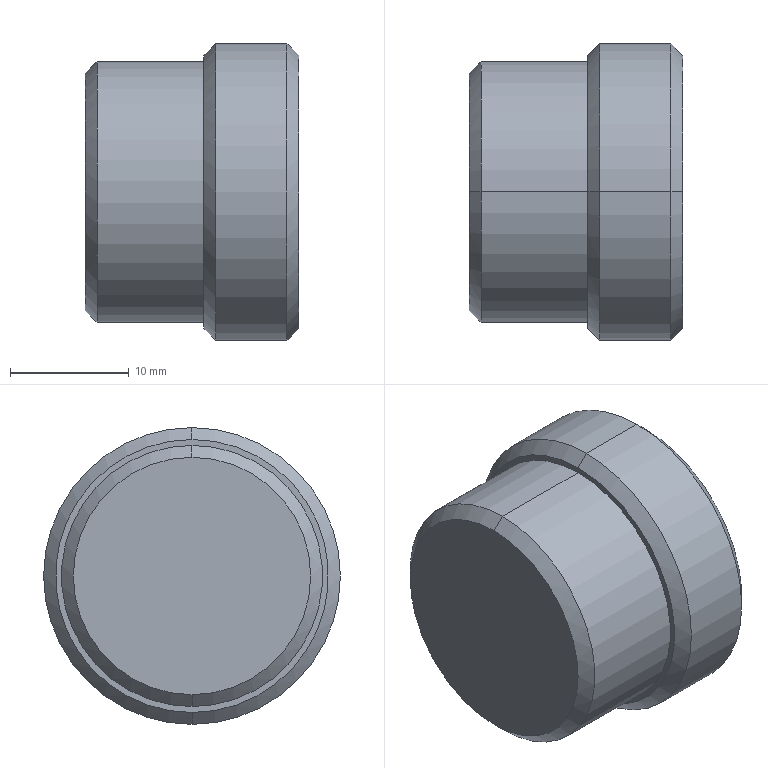Part | STEP file | Panel plug T02 | 1 solid | 13 faces | box 18 x 25 x 25 mm | volume 7618 mm3 | cone 6 | cylinder 4 | plane 3 | commonest cylinder face diameters 22 x2 25 x2
STEP:
#1=CARTESIAN_POINT('',(0.,0.,0.));
#2=DIRECTION('',(0.,0.,1.));
#3=DIRECTION('',(1.,0.,0.));
#4=AXIS2_PLACEMENT_3D('',#1,#2,#3);
#5=CARTESIAN_POINT('',(18.,0.,-11.5));
#6=VERTEX_POINT('',#5);
#7=CARTESIAN_POINT('',(18.,0.,11.5));
#8=VERTEX_POINT('',#7);
#9=CARTESIAN_POINT('',(18.,0.,0.));
#10=DIRECTION('',(1.,0.,0.));
#11=DIRECTION('',(0.,0.,-1.));
#12=AXIS2_PLACEMENT_3D('',#9,#10,#11);
#13=CIRCLE('',#12,11.5);
#14=CARTESIAN_POINT('',(18.,0.,0.));
#15=DIRECTION('',(-1.,0.,0.));
#16=DIRECTION('',(0.,0.,1.));
#17=AXIS2_PLACEMENT_3D('',#14,#15,#16);
#18=CONICAL_SURFACE('',#17,11.5,0.7854);
#19=CARTESIAN_POINT('',(3.142,0.));
#20=DIRECTION('',(-1.,0.));
#21=VECTOR('',#20,1.);
#22=LINE('',#19,#21);
#23=(GEOMETRIC_REPRESENTATION_CONTEXT(2)PARAMETRIC_REPRESENTATION_CONTEXT()REPRESENTATION_CONTEXT('',''));
#24=DEFINITIONAL_REPRESENTATION('',(#22),#23);
#25=PCURVE('',#18,#24);
#26=CARTESIAN_POINT('',(18.,0.,-12.5));
#27=DIRECTION('',(1.,0.,0.));
#28=DIRECTION('',(0.,0.,-1.));
#29=AXIS2_PLACEMENT_3D('',#26,#27,#28);
#30=PLANE('',#29);
#31=CARTESIAN_POINT('',(-12.5,0.));
#32=DIRECTION('',(1.,0.));
#33=AXIS2_PLACEMENT_2D('',#31,#32);
#34=CIRCLE('',#33,11.5);
#35=(GEOMETRIC_REPRESENTATION_CONTEXT(2)PARAMETRIC_REPRESENTATION_CONTEXT()REPRESENTATION_CONTEXT('',''));
#36=DEFINITIONAL_REPRESENTATION('',(#34),#35);
#37=PCURVE('',#30,#36);
#38=SURFACE_CURVE('',#13,(#25,#37),.PCURVE_S1.);
#39=EDGE_CURVE('',#6,#8,#38,.T.);
#40=ORIENTED_EDGE('',*,*,#39,.F.);
#41=CARTESIAN_POINT('',(17.,0.,-12.5));
#42=VERTEX_POINT('',#41);
#43=CARTESIAN_POINT('',(18.,0.,-11.5));
#44=DIRECTION('',(-0.7071,0.,-0.7071));
#45=VECTOR('',#44,1.);
#46=LINE('',#43,#45);
#47=CARTESIAN_POINT('',(3.142,0.));
#48=DIRECTION('',(0.,1.));
#49=VECTOR('',#48,1.);
#50=LINE('',#47,#49);
#51=(GEOMETRIC_REPRESENTATION_CONTEXT(2)PARAMETRIC_REPRESENTATION_CONTEXT()REPRESENTATION_CONTEXT('',''));
#52=DEFINITIONAL_REPRESENTATION('',(#50),#51);
#53=PCURVE('',#18,#52);
#54=CARTESIAN_POINT('',(18.,0.,0.));
#55=DIRECTION('',(-1.,0.,0.));
#56=DIRECTION('',(0.,0.,1.));
#57=AXIS2_PLACEMENT_3D('',#54,#55,#56);
#58=CONICAL_SURFACE('',#57,11.5,0.7854);
#59=CARTESIAN_POINT('',(3.142,0.));
#60=DIRECTION('',(0.,1.));
#61=VECTOR('',#60,1.);
#62=LINE('',#59,#61);
#63=(GEOMETRIC_REPRESENTATION_CONTEXT(2)PARAMETRIC_REPRESENTATION_CONTEXT()REPRESENTATION_CONTEXT('',''));
#64=DEFINITIONAL_REPRESENTATION('',(#62),#63);
#65=PCURVE('',#58,#64);
#66=SURFACE_CURVE('',#46,(#53,#65),.PCURVE_S1.);
#67=EDGE_CURVE('',#6,#42,#66,.T.);
#68=ORIENTED_EDGE('',*,*,#67,.T.);
#69=CARTESIAN_POINT('',(17.,0.,12.5));
#70=VERTEX_POINT('',#69);
#71=CARTESIAN_POINT('',(17.,0.,0.));
#72=DIRECTION('',(-1.,0.,0.));
#73=DIRECTION('',(0.,0.,-1.));
#74=AXIS2_PLACEMENT_3D('',#71,#72,#73);
#75=CIRCLE('',#74,12.5);
#76=CARTESIAN_POINT('',(-3.142,1.));
#77=DIRECTION('',(1.,0.));
#78=VECTOR('',#77,1.);
#79=LINE('',#76,#78);
#80=(GEOMETRIC_REPRESENTATION_CONTEXT(2)PARAMETRIC_REPRESENTATION_CONTEXT()REPRESENTATION_CONTEXT('',''));
#81=DEFINITIONAL_REPRESENTATION('',(#79),#80);
#82=PCURVE('',#18,#81);
#83=CARTESIAN_POINT('',(18.,0.,0.));
#84=DIRECTION('',(1.,0.,0.));
#85=DIRECTION('',(0.,0.,-1.));
#86=AXIS2_PLACEMENT_3D('',#83,#84,#85);
#87=CYLINDRICAL_SURFACE('',#86,12.5);
#88=CARTESIAN_POINT('',(6.283,-1.));
#89=DIRECTION('',(-1.,0.));
#90=VECTOR('',#89,1.);
#91=LINE('',#88,#90);
#92=(GEOMETRIC_REPRESENTATION_CONTEXT(2)PARAMETRIC_REPRESENTATION_CONTEXT()REPRESENTATION_CONTEXT('',''));
#93=DEFINITIONAL_REPRESENTATION('',(#91),#92);
#94=PCURVE('',#87,#93);
#95=SURFACE_CURVE('',#75,(#82,#94),.PCURVE_S1.);
#96=EDGE_CURVE('',#70,#42,#95,.T.);
#97=ORIENTED_EDGE('',*,*,#96,.F.);
#98=CARTESIAN_POINT('',(18.,0.,11.5));
#99=DIRECTION('',(-0.7071,0.,0.7071));
#100=VECTOR('',#99,1.);
#101=LINE('',#98,#100);
#102=CARTESIAN_POINT('',(0.,0.));
#103=DIRECTION('',(0.,1.));
#104=VECTOR('',#103,1.);
#105=LINE('',#102,#104);
#106=(GEOMETRIC_REPRESENTATION_CONTEXT(2)PARAMETRIC_REPRESENTATION_CONTEXT()REPRESENTATION_CONTEXT('',''));
#107=DEFINITIONAL_REPRESENTATION('',(#105),#106);
#108=PCURVE('',#18,#107);
#109=CARTESIAN_POINT('',(6.283,0.));
#110=DIRECTION('',(0.,1.));
#111=VECTOR('',#110,1.);
#112=LINE('',#109,#111);
#113=(GEOMETRIC_REPRESENTATION_CONTEXT(2)PARAMETRIC_REPRESENTATION_CONTEXT()REPRESENTATION_CONTEXT('',''));
#114=DEFINITIONAL_REPRESENTATION('',(#112),#113);
#115=PCURVE('',#58,#114);
#116=SURFACE_CURVE('',#101,(#108,#115),.PCURVE_S1.);
#117=EDGE_CURVE('',#8,#70,#116,.T.);
#118=ORIENTED_EDGE('',*,*,#117,.F.);
#119=EDGE_LOOP('',(#40,#68,#97,#118));
#120=FACE_BOUND('',#119,.T.);
#121=ADVANCED_FACE('',(#120),#18,.T.);
#122=CARTESIAN_POINT('',(10.,0.,11.5));
#123=VERTEX_POINT('',#122);
#124=CARTESIAN_POINT('',(10.,0.,-11.5));
#125=VERTEX_POINT('',#124);
#126=CARTESIAN_POINT('',(10.,0.,0.));
#127=DIRECTION('',(-1.,0.,0.));
#128=DIRECTION('',(0.,0.,1.));
#129=AXIS2_PLACEMENT_3D('',#126,#127,#128);
#130=CIRCLE('',#129,11.5);
#131=CARTESIAN_POINT('',(11.,0.,0.));
#132=DIRECTION('',(1.,0.,0.));
#133=DIRECTION('',(0.,0.,-1.));
#134=AXIS2_PLACEMENT_3D('',#131,#132,#133);
#135=CONICAL_SURFACE('',#134,12.5,0.7854);
#136=CARTESIAN_POINT('',(3.142,-1.));
#137=DIRECTION('',(-1.,0.));
#138=VECTOR('',#137,1.);
#139=LINE('',#136,#138);
#140=(GEOMETRIC_REPRESENTATION_CONTEXT(2)PARAMETRIC_REPRESENTATION_CONTEXT()REPRESENTATION_CONTEXT('',''));
#141=DEFINITIONAL_REPRESENTATION('',(#139),#140);
#142=PCURVE('',#135,#141);
#143=CARTESIAN_POINT('',(10.,0.,-11.));
#144=DIRECTION('',(-1.,0.,0.));
#145=DIRECTION('',(0.,0.,1.));
#146=AXIS2_PLACEMENT_3D('',#143,#144,#145);
#147=PLANE('',#146);
#148=CARTESIAN_POINT('',(11.,0.));
#149=DIRECTION('',(1.,0.));
#150=AXIS2_PLACEMENT_2D('',#148,#149);
#151=CIRCLE('',#150,11.5);
#152=(GEOMETRIC_REPRESENTATION_CONTEXT(2)PARAMETRIC_REPRESENTATION_CONTEXT()REPRESENTATION_CONTEXT('',''));
#153=DEFINITIONAL_REPRESENTATION('',(#151),#152);
#154=PCURVE('',#147,#153);
#155=SURFACE_CURVE('',#130,(#142,#154),.PCURVE_S1.);
#156=EDGE_CURVE('',#123,#125,#155,.T.);
#157=ORIENTED_EDGE('',*,*,#156,.F.);
#158=CARTESIAN_POINT('',(11.,0.,12.5));
#159=VERTEX_POINT('',#158);
#160=CARTESIAN_POINT('',(11.,0.,12.5));
#161=DIRECTION('',(0.7071,0.,0.7071));
#162=VECTOR('',#161,1.);
#163=LINE('',#160,#162);
#164=CARTESIAN_POINT('',(3.142,0.));
#165=DIRECTION('',(0.,1.));
#166=VECTOR('',#165,1.);
#167=LINE('',#164,#166);
#168=(GEOMETRIC_REPRESENTATION_CONTEXT(2)PARAMETRIC_REPRESENTATION_CONTEXT()REPRESENTATION_CONTEXT('',''));
#169=DEFINITIONAL_REPRESENTATION('',(#167),#168);
#170=PCURVE('',#135,#169);
#171=CARTESIAN_POINT('',(11.,0.,0.));
#172=DIRECTION('',(1.,0.,0.));
#173=DIRECTION('',(0.,0.,-1.));
#174=AXIS2_PLACEMENT_3D('',#171,#172,#173);
#175=CONICAL_SURFACE('',#174,12.5,0.7854);
#176=CARTESIAN_POINT('',(3.142,0.));
#177=DIRECTION('',(0.,1.));
#178=VECTOR('',#177,1.);
#179=LINE('',#176,#178);
#180=(GEOMETRIC_REPRESENTATION_CONTEXT(2)PARAMETRIC_REPRESENTATION_CONTEXT()REPRESENTATION_CONTEXT('',''));
#181=DEFINITIONAL_REPRESENTATION('',(#179),#180);
#182=PCURVE('',#175,#181);
#183=SURFACE_CURVE('',#163,(#170,#182),.PCURVE_S1.);
#184=EDGE_CURVE('',#123,#159,#183,.T.);
#185=ORIENTED_EDGE('',*,*,#184,.T.);
#186=CARTESIAN_POINT('',(11.,0.,-12.5));
#187=VERTEX_POINT('',#186);
#188=CARTESIAN_POINT('',(11.,0.,0.));
#189=DIRECTION('',(1.,0.,0.));
#190=DIRECTION('',(0.,0.,1.));
#191=AXIS2_PLACEMENT_3D('',#188,#189,#190);
#192=CIRCLE('',#191,12.5);
#193=CARTESIAN_POINT('',(-3.142,0.));
#194=DIRECTION('',(1.,0.));
#195=VECTOR('',#194,1.);
#196=LINE('',#193,#195);
#197=(GEOMETRIC_REPRESENTATION_CONTEXT(2)PARAMETRIC_REPRESENTATION_CONTEXT()REPRESENTATION_CONTEXT('',''));
#198=DEFINITIONAL_REPRESENTATION('',(#196),#197);
#199=PCURVE('',#135,#198);
#200=CARTESIAN_POINT('',(-3.142,-7.));
#201=DIRECTION('',(1.,0.));
#202=VECTOR('',#201,1.);
#203=LINE('',#200,#202);
#204=(GEOMETRIC_REPRESENTATION_CONTEXT(2)PARAMETRIC_REPRESENTATION_CONTEXT()REPRESENTATION_CONTEXT('',''));
#205=DEFINITIONAL_REPRESENTATION('',(#203),#204);
#206=PCURVE('',#87,#205);
#207=SURFACE_CURVE('',#192,(#199,#206),.PCURVE_S1.);
#208=EDGE_CURVE('',#187,#159,#207,.T.);
#209=ORIENTED_EDGE('',*,*,#208,.F.);
#210=CARTESIAN_POINT('',(11.,0.,-12.5));
#211=DIRECTION('',(0.7071,0.,-0.7071));
#212=VECTOR('',#211,1.);
#213=LINE('',#210,#212);
#214=CARTESIAN_POINT('',(0.,0.));
#215=DIRECTION('',(0.,1.));
#216=VECTOR('',#215,1.);
#217=LINE('',#214,#216);
#218=(GEOMETRIC_REPRESENTATION_CONTEXT(2)PARAMETRIC_REPRESENTATION_CONTEXT()REPRESENTATION_CONTEXT('',''));
#219=DEFINITIONAL_REPRESENTATION('',(#217),#218);
#220=PCURVE('',#135,#219);
#221=CARTESIAN_POINT('',(6.283,0.));
#222=DIRECTION('',(0.,1.));
#223=VECTOR('',#222,1.);
#224=LINE('',#221,#223);
#225=(GEOMETRIC_REPRESENTATION_CONTEXT(2)PARAMETRIC_REPRESENTATION_CONTEXT()REPRESENTATION_CONTEXT('',''));
#226=DEFINITIONAL_REPRESENTATION('',(#224),#225);
#227=PCURVE('',#175,#226);
#228=SURFACE_CURVE('',#213,(#220,#227),.PCURVE_S1.);
#229=EDGE_CURVE('',#125,#187,#228,.T.);
#230=ORIENTED_EDGE('',*,*,#229,.F.);
#231=EDGE_LOOP('',(#157,#185,#209,#230));
#232=FACE_BOUND('',#231,.T.);
#233=ADVANCED_FACE('',(#232),#135,.T.);
#234=CARTESIAN_POINT('',(0.,0.,10.));
#235=VERTEX_POINT('',#234);
#236=CARTESIAN_POINT('',(0.,0.,-10.));
#237=VERTEX_POINT('',#236);
#238=CARTESIAN_POINT('',(0.,0.,0.));
#239=DIRECTION('',(-1.,0.,0.));
#240=DIRECTION('',(0.,0.,1.));
#241=AXIS2_PLACEMENT_3D('',#238,#239,#240);
#242=CIRCLE('',#241,10.);
#243=CARTESIAN_POINT('',(1.,0.,0.));
#244=DIRECTION('',(1.,0.,0.));
#245=DIRECTION('',(0.,0.,-1.));
#246=AXIS2_PLACEMENT_3D('',#243,#244,#245);
#247=CONICAL_SURFACE('',#246,11.,0.7854);
#248=CARTESIAN_POINT('',(3.142,-1.));
#249=DIRECTION('',(-1.,0.));
#250=VECTOR('',#249,1.);
#251=LINE('',#248,#250);
#252=(GEOMETRIC_REPRESENTATION_CONTEXT(2)PARAMETRIC_REPRESENTATION_CONTEXT()REPRESENTATION_CONTEXT('',''));
#253=DEFINITIONAL_REPRESENTATION('',(#251),#252);
#254=PCURVE('',#247,#253);
#255=CARTESIAN_POINT('',(0.,0.,0.));
#256=DIRECTION('',(-1.,0.,0.));
#257=DIRECTION('',(0.,0.,1.));
#258=AXIS2_PLACEMENT_3D('',#255,#256,#257);
#259=PLANE('',#258);
#260=CARTESIAN_POINT('',(0.,0.));
#261=DIRECTION('',(1.,0.));
#262=AXIS2_PLACEMENT_2D('',#260,#261);
#263=CIRCLE('',#262,10.);
#264=(GEOMETRIC_REPRESENTATION_CONTEXT(2)PARAMETRIC_REPRESENTATION_CONTEXT()REPRESENTATION_CONTEXT('',''));
#265=DEFINITIONAL_REPRESENTATION('',(#263),#264);
#266=PCURVE('',#259,#265);
#267=SURFACE_CURVE('',#242,(#254,#266),.PCURVE_S1.);
#268=EDGE_CURVE('',#235,#237,#267,.T.);
#269=ORIENTED_EDGE('',*,*,#268,.F.);
#270=CARTESIAN_POINT('',(1.,0.,11.));
#271=VERTEX_POINT('',#270);
#272=CARTESIAN_POINT('',(1.,0.,11.));
#273=DIRECTION('',(0.7071,0.,0.7071));
#274=VECTOR('',#273,1.);
#275=LINE('',#272,#274);
#276=CARTESIAN_POINT('',(3.142,0.));
#277=DIRECTION('',(0.,1.));
#278=VECTOR('',#277,1.);
#279=LINE('',#276,#278);
#280=(GEOMETRIC_REPRESENTATION_CONTEXT(2)PARAMETRIC_REPRESENTATION_CONTEXT()REPRESENTATION_CONTEXT('',''));
#281=DEFINITIONAL_REPRESENTATION('',(#279),#280);
#282=PCURVE('',#247,#281);
#283=CARTESIAN_POINT('',(1.,0.,0.));
#284=DIRECTION('',(1.,0.,0.));
#285=DIRECTION('',(0.,0.,-1.));
#286=AXIS2_PLACEMENT_3D('',#283,#284,#285);
#287=CONICAL_SURFACE('',#286,11.,0.7854);
#288=CARTESIAN_POINT('',(3.142,0.));
#289=DIRECTION('',(0.,1.));
#290=VECTOR('',#289,1.);
#291=LINE('',#288,#290);
#292=(GEOMETRIC_REPRESENTATION_CONTEXT(2)PARAMETRIC_REPRESENTATION_CONTEXT()REPRESENTATION_CONTEXT('',''));
#293=DEFINITIONAL_REPRESENTATION('',(#291),#292);
#294=PCURVE('',#287,#293);
#295=SURFACE_CURVE('',#275,(#282,#294),.PCURVE_S1.);
#296=EDGE_CURVE('',#235,#271,#295,.T.);
#297=ORIENTED_EDGE('',*,*,#296,.T.);
#298=CARTESIAN_POINT('',(1.,0.,-11.));
#299=VERTEX_POINT('',#298);
#300=CARTESIAN_POINT('',(1.,0.,0.));
#301=DIRECTION('',(1.,0.,0.));
#302=DIRECTION('',(0.,0.,1.));
#303=AXIS2_PLACEMENT_3D('',#300,#301,#302);
#304=CIRCLE('',#303,11.);
#305=CARTESIAN_POINT('',(-3.142,0.));
#306=DIRECTION('',(1.,0.));
#307=VECTOR('',#306,1.);
#308=LINE('',#305,#307);
#309=(GEOMETRIC_REPRESENTATION_CONTEXT(2)PARAMETRIC_REPRESENTATION_CONTEXT()REPRESENTATION_CONTEXT('',''));
#310=DEFINITIONAL_REPRESENTATION('',(#308),#309);
#311=PCURVE('',#247,#310);
#312=CARTESIAN_POINT('',(18.,0.,0.));
#313=DIRECTION('',(1.,0.,0.));
#314=DIRECTION('',(0.,0.,-1.));
#315=AXIS2_PLACEMENT_3D('',#312,#313,#314);
#316=CYLINDRICAL_SURFACE('',#315,11.);
#317=CARTESIAN_POINT('',(-3.142,-17.));
#318=DIRECTION('',(1.,0.));
#319=VECTOR('',#318,1.);
#320=LINE('',#317,#319);
#321=(GEOMETRIC_REPRESENTATION_CONTEXT(2)PARAMETRIC_REPRESENTATION_CONTEXT()REPRESENTATION_CONTEXT('',''));
#322=DEFINITIONAL_REPRESENTATION('',(#320),#321);
#323=PCURVE('',#316,#322);
#324=SURFACE_CURVE('',#304,(#311,#323),.PCURVE_S1.);
#325=EDGE_CURVE('',#299,#271,#324,.T.);
#326=ORIENTED_EDGE('',*,*,#325,.F.);
#327=CARTESIAN_POINT('',(1.,0.,-11.));
#328=DIRECTION('',(0.7071,0.,-0.7071));
#329=VECTOR('',#328,1.);
#330=LINE('',#327,#329);
#331=CARTESIAN_POINT('',(0.,0.));
#332=DIRECTION('',(0.,1.));
#333=VECTOR('',#332,1.);
#334=LINE('',#331,#333);
#335=(GEOMETRIC_REPRESENTATION_CONTEXT(2)PARAMETRIC_REPRESENTATION_CONTEXT()REPRESENTATION_CONTEXT('',''));
#336=DEFINITIONAL_REPRESENTATION('',(#334),#335);
#337=PCURVE('',#247,#336);
#338=CARTESIAN_POINT('',(6.283,0.));
#339=DIRECTION('',(0.,1.));
#340=VECTOR('',#339,1.);
#341=LINE('',#338,#340);
#342=(GEOMETRIC_REPRESENTATION_CONTEXT(2)PARAMETRIC_REPRESENTATION_CONTEXT()REPRESENTATION_CONTEXT('',''));
#343=DEFINITIONAL_REPRESENTATION('',(#341),#342);
#344=PCURVE('',#287,#343);
#345=SURFACE_CURVE('',#330,(#337,#344),.PCURVE_S1.);
#346=EDGE_CURVE('',#237,#299,#345,.T.);
#347=ORIENTED_EDGE('',*,*,#346,.F.);
#348=EDGE_LOOP('',(#269,#297,#326,#347));
#349=FACE_BOUND('',#348,.T.);
#350=ADVANCED_FACE('',(#349),#247,.T.);
#351=ORIENTED_EDGE('',*,*,#208,.T.);
#352=CARTESIAN_POINT('',(18.,0.,12.5));
#353=DIRECTION('',(1.,0.,0.));
#354=VECTOR('',#353,1.);
#355=LINE('',#352,#354);
#356=CARTESIAN_POINT('',(3.142,0.));
#357=DIRECTION('',(0.,1.));
#358=VECTOR('',#357,1.);
#359=LINE('',#356,#358);
#360=(GEOMETRIC_REPRESENTATION_CONTEXT(2)PARAMETRIC_REPRESENTATION_CONTEXT()REPRESENTATION_CONTEXT('',''));
#361=DEFINITIONAL_REPRESENTATION('',(#359),#360);
#362=PCURVE('',#87,#361);
#363=CARTESIAN_POINT('',(18.,0.,0.));
#364=DIRECTION('',(1.,0.,0.));
#365=DIRECTION('',(0.,0.,-1.));
#366=AXIS2_PLACEMENT_3D('',#363,#364,#365);
#367=CYLINDRICAL_SURFACE('',#366,12.5);
#368=CARTESIAN_POINT('',(3.142,0.));
#369=DIRECTION('',(0.,1.));
#370=VECTOR('',#369,1.);
#371=LINE('',#368,#370);
#372=(GEOMETRIC_REPRESENTATION_CONTEXT(2)PARAMETRIC_REPRESENTATION_CONTEXT()REPRESENTATION_CONTEXT('',''));
#373=DEFINITIONAL_REPRESENTATION('',(#371),#372);
#374=PCURVE('',#367,#373);
#375=SURFACE_CURVE('',#355,(#362,#374),.PCURVE_S1.);
#376=EDGE_CURVE('',#159,#70,#375,.T.);
#377=ORIENTED_EDGE('',*,*,#376,.T.);
#378=ORIENTED_EDGE('',*,*,#96,.T.);
#379=CARTESIAN_POINT('',(18.,0.,-12.5));
#380=DIRECTION('',(1.,0.,0.));
#381=VECTOR('',#380,1.);
#382=LINE('',#379,#381);
#383=CARTESIAN_POINT('',(0.,0.));
#384=DIRECTION('',(0.,1.));
#385=VECTOR('',#384,1.);
#386=LINE('',#383,#385);
#387=(GEOMETRIC_REPRESENTATION_CONTEXT(2)PARAMETRIC_REPRESENTATION_CONTEXT()REPRESENTATION_CONTEXT('',''));
#388=DEFINITIONAL_REPRESENTATION('',(#386),#387);
#389=PCURVE('',#87,#388);
#390=CARTESIAN_POINT('',(6.283,0.));
#391=DIRECTION('',(0.,1.));
#392=VECTOR('',#391,1.);
#393=LINE('',#390,#392);
#394=(GEOMETRIC_REPRESENTATION_CONTEXT(2)PARAMETRIC_REPRESENTATION_CONTEXT()REPRESENTATION_CONTEXT('',''));
#395=DEFINITIONAL_REPRESENTATION('',(#393),#394);
#396=PCURVE('',#367,#395);
#397=SURFACE_CURVE('',#382,(#389,#396),.PCURVE_S1.);
#398=EDGE_CURVE('',#187,#42,#397,.T.);
#399=ORIENTED_EDGE('',*,*,#398,.F.);
#400=EDGE_LOOP('',(#351,#377,#378,#399));
#401=FACE_BOUND('',#400,.T.);
#402=ADVANCED_FACE('',(#401),#87,.T.);
#403=ORIENTED_EDGE('',*,*,#325,.T.);
#404=CARTESIAN_POINT('',(10.,0.,11.));
#405=VERTEX_POINT('',#404);
#406=CARTESIAN_POINT('',(18.,0.,11.));
#407=DIRECTION('',(1.,0.,0.));
#408=VECTOR('',#407,1.);
#409=LINE('',#406,#408);
#410=CARTESIAN_POINT('',(3.142,0.));
#411=DIRECTION('',(0.,1.));
#412=VECTOR('',#411,1.);
#413=LINE('',#410,#412);
#414=(GEOMETRIC_REPRESENTATION_CONTEXT(2)PARAMETRIC_REPRESENTATION_CONTEXT()REPRESENTATION_CONTEXT('',''));
#415=DEFINITIONAL_REPRESENTATION('',(#413),#414);
#416=PCURVE('',#316,#415);
#417=CARTESIAN_POINT('',(18.,0.,0.));
#418=DIRECTION('',(1.,0.,0.));
#419=DIRECTION('',(0.,0.,-1.));
#420=AXIS2_PLACEMENT_3D('',#417,#418,#419);
#421=CYLINDRICAL_SURFACE('',#420,11.);
#422=CARTESIAN_POINT('',(3.142,0.));
#423=DIRECTION('',(0.,1.));
#424=VECTOR('',#423,1.);
#425=LINE('',#422,#424);
#426=(GEOMETRIC_REPRESENTATION_CONTEXT(2)PARAMETRIC_REPRESENTATION_CONTEXT()REPRESENTATION_CONTEXT('',''));
#427=DEFINITIONAL_REPRESENTATION('',(#425),#426);
#428=PCURVE('',#421,#427);
#429=SURFACE_CURVE('',#409,(#416,#428),.PCURVE_S1.);
#430=EDGE_CURVE('',#271,#405,#429,.T.);
#431=ORIENTED_EDGE('',*,*,#430,.T.);
#432=CARTESIAN_POINT('',(10.,0.,-11.));
#433=VERTEX_POINT('',#432);
#434=CARTESIAN_POINT('',(10.,0.,0.));
#435=DIRECTION('',(1.,0.,0.));
#436=DIRECTION('',(0.,0.,-1.));
#437=AXIS2_PLACEMENT_3D('',#434,#435,#436);
#438=CIRCLE('',#437,11.);
#439=CARTESIAN_POINT('',(0.,-8.));
#440=DIRECTION('',(1.,0.));
#441=VECTOR('',#440,1.);
#442=LINE('',#439,#441);
#443=(GEOMETRIC_REPRESENTATION_CONTEXT(2)PARAMETRIC_REPRESENTATION_CONTEXT()REPRESENTATION_CONTEXT('',''));
#444=DEFINITIONAL_REPRESENTATION('',(#442),#443);
#445=PCURVE('',#316,#444);
#446=CARTESIAN_POINT('',(0.,0.));
#447=CARTESIAN_POINT('',(0.,19.053));
#448=CARTESIAN_POINT('',(16.5,9.526));
#449=CARTESIAN_POINT('',(33.,0.));
#450=CARTESIAN_POINT('',(16.5,-9.526));
#451=CARTESIAN_POINT('',(0.,-19.053));
#452=CARTESIAN_POINT('',(0.,0.));
#453=(BOUNDED_CURVE()B_SPLINE_CURVE(2,(#446,#447,#448,#449,#450,#451,#452),.UNSPECIFIED.,.T.,.F.)B_SPLINE_CURVE_WITH_KNOTS((1,2,2,2,2,1),(-2.094,0.,2.094,4.189,6.283,8.378),.UNSPECIFIED.)CURVE()GEOMETRIC_REPRESENTATION_ITEM()RATIONAL_B_SPLINE_CURVE((1.,0.5,1.,0.5,1.,0.5,1.))REPRESENTATION_ITEM(''));
#454=(GEOMETRIC_REPRESENTATION_CONTEXT(2)PARAMETRIC_REPRESENTATION_CONTEXT()REPRESENTATION_CONTEXT('',''));
#455=DEFINITIONAL_REPRESENTATION('',(#453),#454);
#456=PCURVE('',#147,#455);
#457=SURFACE_CURVE('',#438,(#445,#456),.PCURVE_S1.);
#458=EDGE_CURVE('',#433,#405,#457,.T.);
#459=ORIENTED_EDGE('',*,*,#458,.F.);
#460=CARTESIAN_POINT('',(18.,0.,-11.));
#461=DIRECTION('',(1.,0.,0.));
#462=VECTOR('',#461,1.);
#463=LINE('',#460,#462);
#464=CARTESIAN_POINT('',(0.,0.));
#465=DIRECTION('',(0.,1.));
#466=VECTOR('',#465,1.);
#467=LINE('',#464,#466);
#468=(GEOMETRIC_REPRESENTATION_CONTEXT(2)PARAMETRIC_REPRESENTATION_CONTEXT()REPRESENTATION_CONTEXT('',''));
#469=DEFINITIONAL_REPRESENTATION('',(#467),#468);
#470=PCURVE('',#316,#469);
#471=CARTESIAN_POINT('',(6.283,0.));
#472=DIRECTION('',(0.,1.));
#473=VECTOR('',#472,1.);
#474=LINE('',#471,#473);
#475=(GEOMETRIC_REPRESENTATION_CONTEXT(2)PARAMETRIC_REPRESENTATION_CONTEXT()REPRESENTATION_CONTEXT('',''));
#476=DEFINITIONAL_REPRESENTATION('',(#474),#475);
#477=PCURVE('',#421,#476);
#478=SURFACE_CURVE('',#463,(#470,#477),.PCURVE_S1.);
#479=EDGE_CURVE('',#299,#433,#478,.T.);
#480=ORIENTED_EDGE('',*,*,#479,.F.);
#481=EDGE_LOOP('',(#403,#431,#459,#480));
#482=FACE_BOUND('',#481,.T.);
#483=ADVANCED_FACE('',(#482),#316,.T.);
#484=CARTESIAN_POINT('',(0.,0.,0.));
#485=DIRECTION('',(-1.,0.,0.));
#486=DIRECTION('',(0.,0.,1.));
#487=AXIS2_PLACEMENT_3D('',#484,#485,#486);
#488=CIRCLE('',#487,10.);
#489=CARTESIAN_POINT('',(0.,0.));
#490=DIRECTION('',(1.,0.));
#491=AXIS2_PLACEMENT_2D('',#489,#490);
#492=CIRCLE('',#491,10.);
#493=(GEOMETRIC_REPRESENTATION_CONTEXT(2)PARAMETRIC_REPRESENTATION_CONTEXT()REPRESENTATION_CONTEXT('',''));
#494=DEFINITIONAL_REPRESENTATION('',(#492),#493);
#495=PCURVE('',#259,#494);
#496=CARTESIAN_POINT('',(9.425,-1.));
#497=DIRECTION('',(-1.,0.));
#498=VECTOR('',#497,1.);
#499=LINE('',#496,#498);
#500=(GEOMETRIC_REPRESENTATION_CONTEXT(2)PARAMETRIC_REPRESENTATION_CONTEXT()REPRESENTATION_CONTEXT('',''));
#501=DEFINITIONAL_REPRESENTATION('',(#499),#500);
#502=PCURVE('',#287,#501);
#503=SURFACE_CURVE('',#488,(#495,#502),.PCURVE_S1.);
#504=EDGE_CURVE('',#237,#235,#503,.T.);
#505=ORIENTED_EDGE('',*,*,#504,.T.);
#506=ORIENTED_EDGE('',*,*,#268,.T.);
#507=EDGE_LOOP('',(#505,#506));
#508=FACE_BOUND('',#507,.T.);
#509=ADVANCED_FACE('',(#508),#259,.T.);
#510=ORIENTED_EDGE('',*,*,#430,.F.);
#511=CARTESIAN_POINT('',(1.,0.,0.));
#512=DIRECTION('',(1.,0.,0.));
#513=DIRECTION('',(0.,0.,1.));
#514=AXIS2_PLACEMENT_3D('',#511,#512,#513);
#515=CIRCLE('',#514,11.);
#516=CARTESIAN_POINT('',(3.142,-17.));
#517=DIRECTION('',(1.,0.));
#518=VECTOR('',#517,1.);
#519=LINE('',#516,#518);
#520=(GEOMETRIC_REPRESENTATION_CONTEXT(2)PARAMETRIC_REPRESENTATION_CONTEXT()REPRESENTATION_CONTEXT('',''));
#521=DEFINITIONAL_REPRESENTATION('',(#519),#520);
#522=PCURVE('',#421,#521);
#523=CARTESIAN_POINT('',(3.142,0.));
#524=DIRECTION('',(1.,0.));
#525=VECTOR('',#524,1.);
#526=LINE('',#523,#525);
#527=(GEOMETRIC_REPRESENTATION_CONTEXT(2)PARAMETRIC_REPRESENTATION_CONTEXT()REPRESENTATION_CONTEXT('',''));
#528=DEFINITIONAL_REPRESENTATION('',(#526),#527);
#529=PCURVE('',#287,#528);
#530=SURFACE_CURVE('',#515,(#522,#529),.PCURVE_S1.);
#531=EDGE_CURVE('',#271,#299,#530,.T.);
#532=ORIENTED_EDGE('',*,*,#531,.T.);
#533=ORIENTED_EDGE('',*,*,#479,.T.);
#534=CARTESIAN_POINT('',(10.,0.,0.));
#535=DIRECTION('',(1.,0.,0.));
#536=DIRECTION('',(0.,0.,-1.));
#537=AXIS2_PLACEMENT_3D('',#534,#535,#536);
#538=CIRCLE('',#537,11.);
#539=CARTESIAN_POINT('',(0.,-8.));
#540=DIRECTION('',(1.,0.));
#541=VECTOR('',#540,1.);
#542=LINE('',#539,#541);
#543=(GEOMETRIC_REPRESENTATION_CONTEXT(2)PARAMETRIC_REPRESENTATION_CONTEXT()REPRESENTATION_CONTEXT('',''));
#544=DEFINITIONAL_REPRESENTATION('',(#542),#543);
#545=PCURVE('',#421,#544);
#546=CARTESIAN_POINT('',(0.,0.));
#547=CARTESIAN_POINT('',(0.,19.053));
#548=CARTESIAN_POINT('',(16.5,9.526));
#549=CARTESIAN_POINT('',(33.,0.));
#550=CARTESIAN_POINT('',(16.5,-9.526));
#551=CARTESIAN_POINT('',(0.,-19.053));
#552=CARTESIAN_POINT('',(0.,0.));
#553=(BOUNDED_CURVE()B_SPLINE_CURVE(2,(#546,#547,#548,#549,#550,#551,#552),.UNSPECIFIED.,.T.,.F.)B_SPLINE_CURVE_WITH_KNOTS((1,2,2,2,2,1),(-2.094,0.,2.094,4.189,6.283,8.378),.UNSPECIFIED.)CURVE()GEOMETRIC_REPRESENTATION_ITEM()RATIONAL_B_SPLINE_CURVE((1.,0.5,1.,0.5,1.,0.5,1.))REPRESENTATION_ITEM(''));
#554=(GEOMETRIC_REPRESENTATION_CONTEXT(2)PARAMETRIC_REPRESENTATION_CONTEXT()REPRESENTATION_CONTEXT('',''));
#555=DEFINITIONAL_REPRESENTATION('',(#553),#554);
#556=PCURVE('',#147,#555);
#557=SURFACE_CURVE('',#538,(#545,#556),.PCURVE_S1.);
#558=EDGE_CURVE('',#405,#433,#557,.T.);
#559=ORIENTED_EDGE('',*,*,#558,.F.);
#560=EDGE_LOOP('',(#510,#532,#533,#559));
#561=FACE_BOUND('',#560,.T.);
#562=ADVANCED_FACE('',(#561),#421,.T.);
#563=CARTESIAN_POINT('',(10.,0.,0.));
#564=DIRECTION('',(-1.,0.,0.));
#565=DIRECTION('',(0.,0.,1.));
#566=AXIS2_PLACEMENT_3D('',#563,#564,#565);
#567=CIRCLE('',#566,11.5);
#568=CARTESIAN_POINT('',(11.,0.));
#569=DIRECTION('',(1.,0.));
#570=AXIS2_PLACEMENT_2D('',#568,#569);
#571=CIRCLE('',#570,11.5);
#572=(GEOMETRIC_REPRESENTATION_CONTEXT(2)PARAMETRIC_REPRESENTATION_CONTEXT()REPRESENTATION_CONTEXT('',''));
#573=DEFINITIONAL_REPRESENTATION('',(#571),#572);
#574=PCURVE('',#147,#573);
#575=CARTESIAN_POINT('',(9.425,-1.));
#576=DIRECTION('',(-1.,0.));
#577=VECTOR('',#576,1.);
#578=LINE('',#575,#577);
#579=(GEOMETRIC_REPRESENTATION_CONTEXT(2)PARAMETRIC_REPRESENTATION_CONTEXT()REPRESENTATION_CONTEXT('',''));
#580=DEFINITIONAL_REPRESENTATION('',(#578),#579);
#581=PCURVE('',#175,#580);
#582=SURFACE_CURVE('',#567,(#574,#581),.PCURVE_S1.);
#583=EDGE_CURVE('',#125,#123,#582,.T.);
#584=ORIENTED_EDGE('',*,*,#583,.T.);
#585=ORIENTED_EDGE('',*,*,#156,.T.);
#586=EDGE_LOOP('',(#584,#585));
#587=FACE_BOUND('',#586,.T.);
#588=ORIENTED_EDGE('',*,*,#458,.T.);
#589=ORIENTED_EDGE('',*,*,#558,.T.);
#590=EDGE_LOOP('',(#588,#589));
#591=FACE_BOUND('',#590,.T.);
#592=ADVANCED_FACE('',(#587,#591),#147,.T.);
#593=ORIENTED_EDGE('',*,*,#376,.F.);
#594=CARTESIAN_POINT('',(11.,0.,0.));
#595=DIRECTION('',(1.,0.,0.));
#596=DIRECTION('',(0.,0.,1.));
#597=AXIS2_PLACEMENT_3D('',#594,#595,#596);
#598=CIRCLE('',#597,12.5);
#599=CARTESIAN_POINT('',(3.142,-7.));
#600=DIRECTION('',(1.,0.));
#601=VECTOR('',#600,1.);
#602=LINE('',#599,#601);
#603=(GEOMETRIC_REPRESENTATION_CONTEXT(2)PARAMETRIC_REPRESENTATION_CONTEXT()REPRESENTATION_CONTEXT('',''));
#604=DEFINITIONAL_REPRESENTATION('',(#602),#603);
#605=PCURVE('',#367,#604);
#606=CARTESIAN_POINT('',(3.142,0.));
#607=DIRECTION('',(1.,0.));
#608=VECTOR('',#607,1.);
#609=LINE('',#606,#608);
#610=(GEOMETRIC_REPRESENTATION_CONTEXT(2)PARAMETRIC_REPRESENTATION_CONTEXT()REPRESENTATION_CONTEXT('',''));
#611=DEFINITIONAL_REPRESENTATION('',(#609),#610);
#612=PCURVE('',#175,#611);
#613=SURFACE_CURVE('',#598,(#605,#612),.PCURVE_S1.);
#614=EDGE_CURVE('',#159,#187,#613,.T.);
#615=ORIENTED_EDGE('',*,*,#614,.T.);
#616=ORIENTED_EDGE('',*,*,#398,.T.);
#617=CARTESIAN_POINT('',(17.,0.,0.));
#618=DIRECTION('',(-1.,0.,0.));
#619=DIRECTION('',(0.,0.,-1.));
#620=AXIS2_PLACEMENT_3D('',#617,#618,#619);
#621=CIRCLE('',#620,12.5);
#622=CARTESIAN_POINT('',(6.283,-1.));
#623=DIRECTION('',(-1.,0.));
#624=VECTOR('',#623,1.);
#625=LINE('',#622,#624);
#626=(GEOMETRIC_REPRESENTATION_CONTEXT(2)PARAMETRIC_REPRESENTATION_CONTEXT()REPRESENTATION_CONTEXT('',''));
#627=DEFINITIONAL_REPRESENTATION('',(#625),#626);
#628=PCURVE('',#367,#627);
#629=CARTESIAN_POINT('',(3.142,1.));
#630=DIRECTION('',(1.,0.));
#631=VECTOR('',#630,1.);
#632=LINE('',#629,#631);
#633=(GEOMETRIC_REPRESENTATION_CONTEXT(2)PARAMETRIC_REPRESENTATION_CONTEXT()REPRESENTATION_CONTEXT('',''));
#634=DEFINITIONAL_REPRESENTATION('',(#632),#633);
#635=PCURVE('',#58,#634);
#636=SURFACE_CURVE('',#621,(#628,#635),.PCURVE_S1.);
#637=EDGE_CURVE('',#42,#70,#636,.T.);
#638=ORIENTED_EDGE('',*,*,#637,.T.);
#639=EDGE_LOOP('',(#593,#615,#616,#638));
#640=FACE_BOUND('',#639,.T.);
#641=ADVANCED_FACE('',(#640),#367,.T.);
#642=CARTESIAN_POINT('',(18.,0.,0.));
#643=DIRECTION('',(1.,0.,0.));
#644=DIRECTION('',(0.,0.,-1.));
#645=AXIS2_PLACEMENT_3D('',#642,#643,#644);
#646=CIRCLE('',#645,11.5);
#647=CARTESIAN_POINT('',(-12.5,0.));
#648=DIRECTION('',(1.,0.));
#649=AXIS2_PLACEMENT_2D('',#647,#648);
#650=CIRCLE('',#649,11.5);
#651=(GEOMETRIC_REPRESENTATION_CONTEXT(2)PARAMETRIC_REPRESENTATION_CONTEXT()REPRESENTATION_CONTEXT('',''));
#652=DEFINITIONAL_REPRESENTATION('',(#650),#651);
#653=PCURVE('',#30,#652);
#654=CARTESIAN_POINT('',(9.425,0.));
#655=DIRECTION('',(-1.,0.));
#656=VECTOR('',#655,1.);
#657=LINE('',#654,#656);
#658=(GEOMETRIC_REPRESENTATION_CONTEXT(2)PARAMETRIC_REPRESENTATION_CONTEXT()REPRESENTATION_CONTEXT('',''));
#659=DEFINITIONAL_REPRESENTATION('',(#657),#658);
#660=PCURVE('',#58,#659);
#661=SURFACE_CURVE('',#646,(#653,#660),.PCURVE_S1.);
#662=EDGE_CURVE('',#8,#6,#661,.T.);
#663=ORIENTED_EDGE('',*,*,#662,.T.);
#664=ORIENTED_EDGE('',*,*,#39,.T.);
#665=EDGE_LOOP('',(#663,#664));
#666=FACE_BOUND('',#665,.T.);
#667=ADVANCED_FACE('',(#666),#30,.T.);
#668=ORIENTED_EDGE('',*,*,#296,.F.);
#669=ORIENTED_EDGE('',*,*,#504,.F.);
#670=ORIENTED_EDGE('',*,*,#346,.T.);
#671=ORIENTED_EDGE('',*,*,#531,.F.);
#672=EDGE_LOOP('',(#668,#669,#670,#671));
#673=FACE_BOUND('',#672,.T.);
#674=ADVANCED_FACE('',(#673),#287,.T.);
#675=ORIENTED_EDGE('',*,*,#184,.F.);
#676=ORIENTED_EDGE('',*,*,#583,.F.);
#677=ORIENTED_EDGE('',*,*,#229,.T.);
#678=ORIENTED_EDGE('',*,*,#614,.F.);
#679=EDGE_LOOP('',(#675,#676,#677,#678));
#680=FACE_BOUND('',#679,.T.);
#681=ADVANCED_FACE('',(#680),#175,.T.);
#682=ORIENTED_EDGE('',*,*,#67,.F.);
#683=ORIENTED_EDGE('',*,*,#662,.F.);
#684=ORIENTED_EDGE('',*,*,#117,.T.);
#685=ORIENTED_EDGE('',*,*,#637,.F.);
#686=EDGE_LOOP('',(#682,#683,#684,#685));
#687=FACE_BOUND('',#686,.T.);
#688=ADVANCED_FACE('',(#687),#58,.T.);
#689=CLOSED_SHELL('',(#121,#233,#350,#402,#483,#509,#562,#592,#641,#667,#674,#681,#688));
#690=MANIFOLD_SOLID_BREP('',#689);
#691=(LENGTH_UNIT()NAMED_UNIT(*)SI_UNIT(.MILLI.,.METRE.));
#692=UNCERTAINTY_MEASURE_WITH_UNIT(LENGTH_MEASURE(0.0000001),#691,'','');
#693=(NAMED_UNIT(*)PLANE_ANGLE_UNIT()SI_UNIT($,.RADIAN.));
#694=(NAMED_UNIT(*)SI_UNIT($,.STERADIAN.)SOLID_ANGLE_UNIT());
#695=(GEOMETRIC_REPRESENTATION_CONTEXT(3)GLOBAL_UNCERTAINTY_ASSIGNED_CONTEXT((#692))GLOBAL_UNIT_ASSIGNED_CONTEXT((#691,#693,#694))REPRESENTATION_CONTEXT('',''));
#696=ADVANCED_BREP_SHAPE_REPRESENTATION('',(#4,#690),#695);